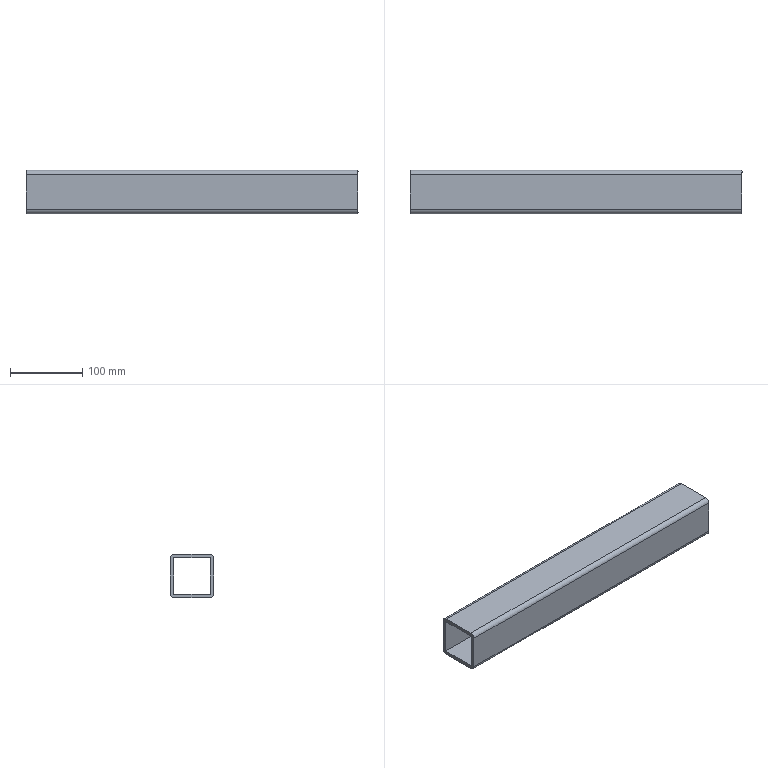Part | STEP file | Positioning_id714_x_t | 1 solid | 14 faces | box 460 x 60 x 60 mm | volume 491785 mm3 | plane 10 | cylinder 4 | commonest cylinder face diameters 12 x4
STEP:
#1=CARTESIAN_POINT('',(0.,0.,0.));
#2=DIRECTION('',(0.,0.,1.));
#3=DIRECTION('',(1.,0.,0.));
#4=AXIS2_PLACEMENT_3D('',#1,#2,#3);
#5=CARTESIAN_POINT('',(-1493.002,-815.,157.466));
#6=VERTEX_POINT('',#5);
#7=CARTESIAN_POINT('',(-1493.002,-765.,157.466));
#8=VERTEX_POINT('',#7);
#9=CARTESIAN_POINT('',(-1493.002,-815.,157.466));
#10=DIRECTION('',(0.,1.,0.));
#11=VECTOR('',#10,1.);
#12=LINE('',#9,#11);
#13=CARTESIAN_POINT('',(-1493.002,-200.,108.466));
#14=DIRECTION('',(1.,0.,0.));
#15=DIRECTION('',(0.,0.,1.));
#16=AXIS2_PLACEMENT_3D('',#13,#14,#15);
#17=PLANE('',#16);
#18=CARTESIAN_POINT('',(49.,615.));
#19=DIRECTION('',(0.,-1.));
#20=VECTOR('',#19,1.);
#21=LINE('',#18,#20);
#22=(GEOMETRIC_REPRESENTATION_CONTEXT(2)PARAMETRIC_REPRESENTATION_CONTEXT()REPRESENTATION_CONTEXT('',''));
#23=DEFINITIONAL_REPRESENTATION('',(#21),#22);
#24=PCURVE('',#17,#23);
#25=CARTESIAN_POINT('',(-1148.002,-815.,157.466));
#26=DIRECTION('',(0.,0.,1.));
#27=DIRECTION('',(0.,1.,0.));
#28=AXIS2_PLACEMENT_3D('',#25,#26,#27);
#29=PLANE('',#28);
#30=CARTESIAN_POINT('',(0.,345.));
#31=DIRECTION('',(1.,0.));
#32=VECTOR('',#31,1.);
#33=LINE('',#30,#32);
#34=(GEOMETRIC_REPRESENTATION_CONTEXT(2)PARAMETRIC_REPRESENTATION_CONTEXT()REPRESENTATION_CONTEXT('',''));
#35=DEFINITIONAL_REPRESENTATION('',(#33),#34);
#36=PCURVE('',#29,#35);
#37=SURFACE_CURVE('',#12,(#24,#36),.PCURVE_S1.);
#38=EDGE_CURVE('',#6,#8,#37,.T.);
#39=ORIENTED_EDGE('',*,*,#38,.F.);
#40=CARTESIAN_POINT('',(-1493.002,-815.,107.466));
#41=VERTEX_POINT('',#40);
#42=CARTESIAN_POINT('',(-1493.002,-815.,107.466));
#43=DIRECTION('',(0.,0.,1.));
#44=VECTOR('',#43,1.);
#45=LINE('',#42,#44);
#46=CARTESIAN_POINT('',(-1.,615.));
#47=DIRECTION('',(1.,0.));
#48=VECTOR('',#47,1.);
#49=LINE('',#46,#48);
#50=(GEOMETRIC_REPRESENTATION_CONTEXT(2)PARAMETRIC_REPRESENTATION_CONTEXT()REPRESENTATION_CONTEXT('',''));
#51=DEFINITIONAL_REPRESENTATION('',(#49),#50);
#52=PCURVE('',#17,#51);
#53=CARTESIAN_POINT('',(-1148.002,-815.,132.466));
#54=DIRECTION('',(0.,-1.,0.));
#55=DIRECTION('',(0.,0.,1.));
#56=AXIS2_PLACEMENT_3D('',#53,#54,#55);
#57=PLANE('',#56);
#58=CARTESIAN_POINT('',(-25.,345.));
#59=DIRECTION('',(1.,0.));
#60=VECTOR('',#59,1.);
#61=LINE('',#58,#60);
#62=(GEOMETRIC_REPRESENTATION_CONTEXT(2)PARAMETRIC_REPRESENTATION_CONTEXT()REPRESENTATION_CONTEXT('',''));
#63=DEFINITIONAL_REPRESENTATION('',(#61),#62);
#64=PCURVE('',#57,#63);
#65=SURFACE_CURVE('',#45,(#52,#64),.PCURVE_S1.);
#66=EDGE_CURVE('',#41,#6,#65,.T.);
#67=ORIENTED_EDGE('',*,*,#66,.F.);
#68=CARTESIAN_POINT('',(-1493.002,-765.,107.466));
#69=VERTEX_POINT('',#68);
#70=CARTESIAN_POINT('',(-1493.002,-765.,107.466));
#71=DIRECTION('',(0.,-1.,0.));
#72=VECTOR('',#71,1.);
#73=LINE('',#70,#72);
#74=CARTESIAN_POINT('',(-1.,565.));
#75=DIRECTION('',(0.,1.));
#76=VECTOR('',#75,1.);
#77=LINE('',#74,#76);
#78=(GEOMETRIC_REPRESENTATION_CONTEXT(2)PARAMETRIC_REPRESENTATION_CONTEXT()REPRESENTATION_CONTEXT('',''));
#79=DEFINITIONAL_REPRESENTATION('',(#77),#78);
#80=PCURVE('',#17,#79);
#81=CARTESIAN_POINT('',(-1148.002,-815.,107.466));
#82=DIRECTION('',(0.,0.,-1.));
#83=DIRECTION('',(0.,-1.,0.));
#84=AXIS2_PLACEMENT_3D('',#81,#82,#83);
#85=PLANE('',#84);
#86=CARTESIAN_POINT('',(-50.,345.));
#87=DIRECTION('',(1.,0.));
#88=VECTOR('',#87,1.);
#89=LINE('',#86,#88);
#90=(GEOMETRIC_REPRESENTATION_CONTEXT(2)PARAMETRIC_REPRESENTATION_CONTEXT()REPRESENTATION_CONTEXT('',''));
#91=DEFINITIONAL_REPRESENTATION('',(#89),#90);
#92=PCURVE('',#85,#91);
#93=SURFACE_CURVE('',#73,(#80,#92),.PCURVE_S1.);
#94=EDGE_CURVE('',#69,#41,#93,.T.);
#95=ORIENTED_EDGE('',*,*,#94,.F.);
#96=CARTESIAN_POINT('',(-1493.002,-765.,157.466));
#97=DIRECTION('',(0.,0.,-1.));
#98=VECTOR('',#97,1.);
#99=LINE('',#96,#98);
#100=CARTESIAN_POINT('',(49.,565.));
#101=DIRECTION('',(-1.,0.));
#102=VECTOR('',#101,1.);
#103=LINE('',#100,#102);
#104=(GEOMETRIC_REPRESENTATION_CONTEXT(2)PARAMETRIC_REPRESENTATION_CONTEXT()REPRESENTATION_CONTEXT('',''));
#105=DEFINITIONAL_REPRESENTATION('',(#103),#104);
#106=PCURVE('',#17,#105);
#107=CARTESIAN_POINT('',(-1148.002,-765.,132.466));
#108=DIRECTION('',(0.,1.,0.));
#109=DIRECTION('',(0.,0.,-1.));
#110=AXIS2_PLACEMENT_3D('',#107,#108,#109);
#111=PLANE('',#110);
#112=CARTESIAN_POINT('',(-25.,345.));
#113=DIRECTION('',(1.,0.));
#114=VECTOR('',#113,1.);
#115=LINE('',#112,#114);
#116=(GEOMETRIC_REPRESENTATION_CONTEXT(2)PARAMETRIC_REPRESENTATION_CONTEXT()REPRESENTATION_CONTEXT('',''));
#117=DEFINITIONAL_REPRESENTATION('',(#115),#116);
#118=PCURVE('',#111,#117);
#119=SURFACE_CURVE('',#99,(#106,#118),.PCURVE_S1.);
#120=EDGE_CURVE('',#8,#69,#119,.T.);
#121=ORIENTED_EDGE('',*,*,#120,.F.);
#122=EDGE_LOOP('',(#39,#67,#95,#121));
#123=FACE_BOUND('',#122,.T.);
#124=CARTESIAN_POINT('',(-1493.002,-760.,108.466));
#125=VERTEX_POINT('',#124);
#126=CARTESIAN_POINT('',(-1493.002,-766.,102.466));
#127=VERTEX_POINT('',#126);
#128=CARTESIAN_POINT('',(-1493.002,-766.,108.466));
#129=DIRECTION('',(-1.,0.,0.));
#130=DIRECTION('',(0.,1.,0.));
#131=AXIS2_PLACEMENT_3D('',#128,#129,#130);
#132=CIRCLE('',#131,6.);
#133=CARTESIAN_POINT('',(0.,560.));
#134=CARTESIAN_POINT('',(-10.392,560.));
#135=CARTESIAN_POINT('',(-5.196,569.));
#136=CARTESIAN_POINT('',(0.,578.));
#137=CARTESIAN_POINT('',(5.196,569.));
#138=CARTESIAN_POINT('',(10.392,560.));
#139=CARTESIAN_POINT('',(0.,560.));
#140=(BOUNDED_CURVE()B_SPLINE_CURVE(2,(#133,#134,#135,#136,#137,#138,#139),.UNSPECIFIED.,.T.,.F.)B_SPLINE_CURVE_WITH_KNOTS((1,2,2,2,2,1),(-2.094,0.,2.094,4.189,6.283,8.378),.UNSPECIFIED.)CURVE()GEOMETRIC_REPRESENTATION_ITEM()RATIONAL_B_SPLINE_CURVE((1.,0.5,1.,0.5,1.,0.5,1.))REPRESENTATION_ITEM(''));
#141=(GEOMETRIC_REPRESENTATION_CONTEXT(2)PARAMETRIC_REPRESENTATION_CONTEXT()REPRESENTATION_CONTEXT('',''));
#142=DEFINITIONAL_REPRESENTATION('',(#140),#141);
#143=PCURVE('',#17,#142);
#144=CARTESIAN_POINT('',(-1148.002,-766.,108.466));
#145=DIRECTION('',(-1.,0.,0.));
#146=DIRECTION('',(0.,0.,1.));
#147=AXIS2_PLACEMENT_3D('',#144,#145,#146);
#148=CYLINDRICAL_SURFACE('',#147,6.);
#149=CARTESIAN_POINT('',(1.571,345.));
#150=DIRECTION('',(1.,0.));
#151=VECTOR('',#150,1.);
#152=LINE('',#149,#151);
#153=(GEOMETRIC_REPRESENTATION_CONTEXT(2)PARAMETRIC_REPRESENTATION_CONTEXT()REPRESENTATION_CONTEXT('',''));
#154=DEFINITIONAL_REPRESENTATION('',(#152),#153);
#155=PCURVE('',#148,#154);
#156=SURFACE_CURVE('',#132,(#143,#155),.PCURVE_S1.);
#157=EDGE_CURVE('',#125,#127,#156,.T.);
#158=ORIENTED_EDGE('',*,*,#157,.T.);
#159=CARTESIAN_POINT('',(-1493.002,-814.,102.466));
#160=VERTEX_POINT('',#159);
#161=CARTESIAN_POINT('',(-1493.002,-766.,102.466));
#162=DIRECTION('',(0.,-1.,0.));
#163=VECTOR('',#162,1.);
#164=LINE('',#161,#163);
#165=CARTESIAN_POINT('',(-6.,566.));
#166=DIRECTION('',(0.,1.));
#167=VECTOR('',#166,1.);
#168=LINE('',#165,#167);
#169=(GEOMETRIC_REPRESENTATION_CONTEXT(2)PARAMETRIC_REPRESENTATION_CONTEXT()REPRESENTATION_CONTEXT('',''));
#170=DEFINITIONAL_REPRESENTATION('',(#168),#169);
#171=PCURVE('',#17,#170);
#172=CARTESIAN_POINT('',(-1148.002,-820.,102.466));
#173=DIRECTION('',(0.,0.,-1.));
#174=DIRECTION('',(0.,-1.,0.));
#175=AXIS2_PLACEMENT_3D('',#172,#173,#174);
#176=PLANE('',#175);
#177=CARTESIAN_POINT('',(-54.,345.));
#178=DIRECTION('',(1.,0.));
#179=VECTOR('',#178,1.);
#180=LINE('',#177,#179);
#181=(GEOMETRIC_REPRESENTATION_CONTEXT(2)PARAMETRIC_REPRESENTATION_CONTEXT()REPRESENTATION_CONTEXT('',''));
#182=DEFINITIONAL_REPRESENTATION('',(#180),#181);
#183=PCURVE('',#176,#182);
#184=SURFACE_CURVE('',#164,(#171,#183),.PCURVE_S1.);
#185=EDGE_CURVE('',#127,#160,#184,.T.);
#186=ORIENTED_EDGE('',*,*,#185,.T.);
#187=CARTESIAN_POINT('',(-1493.002,-820.,108.466));
#188=VERTEX_POINT('',#187);
#189=CARTESIAN_POINT('',(-1493.002,-814.,108.466));
#190=DIRECTION('',(-1.,0.,0.));
#191=DIRECTION('',(0.,0.,-1.));
#192=AXIS2_PLACEMENT_3D('',#189,#190,#191);
#193=CIRCLE('',#192,6.);
#194=CARTESIAN_POINT('',(-6.,614.));
#195=CARTESIAN_POINT('',(-6.,624.392));
#196=CARTESIAN_POINT('',(3.,619.196));
#197=CARTESIAN_POINT('',(12.,614.));
#198=CARTESIAN_POINT('',(3.,608.804));
#199=CARTESIAN_POINT('',(-6.,603.608));
#200=CARTESIAN_POINT('',(-6.,614.));
#201=(BOUNDED_CURVE()B_SPLINE_CURVE(2,(#194,#195,#196,#197,#198,#199,#200),.UNSPECIFIED.,.T.,.F.)B_SPLINE_CURVE_WITH_KNOTS((1,2,2,2,2,1),(-2.094,0.,2.094,4.189,6.283,8.378),.UNSPECIFIED.)CURVE()GEOMETRIC_REPRESENTATION_ITEM()RATIONAL_B_SPLINE_CURVE((1.,0.5,1.,0.5,1.,0.5,1.))REPRESENTATION_ITEM(''));
#202=(GEOMETRIC_REPRESENTATION_CONTEXT(2)PARAMETRIC_REPRESENTATION_CONTEXT()REPRESENTATION_CONTEXT('',''));
#203=DEFINITIONAL_REPRESENTATION('',(#201),#202);
#204=PCURVE('',#17,#203);
#205=CARTESIAN_POINT('',(-1148.002,-814.,108.466));
#206=DIRECTION('',(1.,0.,0.));
#207=DIRECTION('',(0.,0.,-1.));
#208=AXIS2_PLACEMENT_3D('',#205,#206,#207);
#209=CYLINDRICAL_SURFACE('',#208,6.);
#210=CARTESIAN_POINT('',(6.283,-345.));
#211=DIRECTION('',(-1.,0.));
#212=VECTOR('',#211,1.);
#213=LINE('',#210,#212);
#214=(GEOMETRIC_REPRESENTATION_CONTEXT(2)PARAMETRIC_REPRESENTATION_CONTEXT()REPRESENTATION_CONTEXT('',''));
#215=DEFINITIONAL_REPRESENTATION('',(#213),#214);
#216=PCURVE('',#209,#215);
#217=SURFACE_CURVE('',#193,(#204,#216),.PCURVE_S1.);
#218=EDGE_CURVE('',#160,#188,#217,.T.);
#219=ORIENTED_EDGE('',*,*,#218,.T.);
#220=CARTESIAN_POINT('',(-1493.002,-820.,156.466));
#221=VERTEX_POINT('',#220);
#222=CARTESIAN_POINT('',(-1493.002,-820.,108.466));
#223=DIRECTION('',(0.,0.,1.));
#224=VECTOR('',#223,1.);
#225=LINE('',#222,#224);
#226=CARTESIAN_POINT('',(0.,620.));
#227=DIRECTION('',(1.,0.));
#228=VECTOR('',#227,1.);
#229=LINE('',#226,#228);
#230=(GEOMETRIC_REPRESENTATION_CONTEXT(2)PARAMETRIC_REPRESENTATION_CONTEXT()REPRESENTATION_CONTEXT('',''));
#231=DEFINITIONAL_REPRESENTATION('',(#229),#230);
#232=PCURVE('',#17,#231);
#233=CARTESIAN_POINT('',(-1148.002,-820.,132.466));
#234=DIRECTION('',(0.,-1.,0.));
#235=DIRECTION('',(0.,0.,1.));
#236=AXIS2_PLACEMENT_3D('',#233,#234,#235);
#237=PLANE('',#236);
#238=CARTESIAN_POINT('',(-24.,345.));
#239=DIRECTION('',(1.,0.));
#240=VECTOR('',#239,1.);
#241=LINE('',#238,#240);
#242=(GEOMETRIC_REPRESENTATION_CONTEXT(2)PARAMETRIC_REPRESENTATION_CONTEXT()REPRESENTATION_CONTEXT('',''));
#243=DEFINITIONAL_REPRESENTATION('',(#241),#242);
#244=PCURVE('',#237,#243);
#245=SURFACE_CURVE('',#225,(#232,#244),.PCURVE_S1.);
#246=EDGE_CURVE('',#188,#221,#245,.T.);
#247=ORIENTED_EDGE('',*,*,#246,.T.);
#248=CARTESIAN_POINT('',(-1493.002,-814.,162.466));
#249=VERTEX_POINT('',#248);
#250=CARTESIAN_POINT('',(-1493.002,-814.,156.466));
#251=DIRECTION('',(-1.,0.,0.));
#252=DIRECTION('',(0.,-1.,0.));
#253=AXIS2_PLACEMENT_3D('',#250,#251,#252);
#254=CIRCLE('',#253,6.);
#255=CARTESIAN_POINT('',(48.,620.));
#256=CARTESIAN_POINT('',(58.392,620.));
#257=CARTESIAN_POINT('',(53.196,611.));
#258=CARTESIAN_POINT('',(48.,602.));
#259=CARTESIAN_POINT('',(42.804,611.));
#260=CARTESIAN_POINT('',(37.608,620.));
#261=CARTESIAN_POINT('',(48.,620.));
#262=(BOUNDED_CURVE()B_SPLINE_CURVE(2,(#255,#256,#257,#258,#259,#260,#261),.UNSPECIFIED.,.T.,.F.)B_SPLINE_CURVE_WITH_KNOTS((1,2,2,2,2,1),(-2.094,0.,2.094,4.189,6.283,8.378),.UNSPECIFIED.)CURVE()GEOMETRIC_REPRESENTATION_ITEM()RATIONAL_B_SPLINE_CURVE((1.,0.5,1.,0.5,1.,0.5,1.))REPRESENTATION_ITEM(''));
#263=(GEOMETRIC_REPRESENTATION_CONTEXT(2)PARAMETRIC_REPRESENTATION_CONTEXT()REPRESENTATION_CONTEXT('',''));
#264=DEFINITIONAL_REPRESENTATION('',(#262),#263);
#265=PCURVE('',#17,#264);
#266=CARTESIAN_POINT('',(-1148.002,-814.,156.466));
#267=DIRECTION('',(-1.,0.,0.));
#268=DIRECTION('',(0.,0.,1.));
#269=AXIS2_PLACEMENT_3D('',#266,#267,#268);
#270=CYLINDRICAL_SURFACE('',#269,6.);
#271=CARTESIAN_POINT('',(4.712,345.));
#272=DIRECTION('',(1.,0.));
#273=VECTOR('',#272,1.);
#274=LINE('',#271,#273);
#275=(GEOMETRIC_REPRESENTATION_CONTEXT(2)PARAMETRIC_REPRESENTATION_CONTEXT()REPRESENTATION_CONTEXT('',''));
#276=DEFINITIONAL_REPRESENTATION('',(#274),#275);
#277=PCURVE('',#270,#276);
#278=SURFACE_CURVE('',#254,(#265,#277),.PCURVE_S1.);
#279=EDGE_CURVE('',#221,#249,#278,.T.);
#280=ORIENTED_EDGE('',*,*,#279,.T.);
#281=CARTESIAN_POINT('',(-1493.002,-766.,162.466));
#282=VERTEX_POINT('',#281);
#283=CARTESIAN_POINT('',(-1493.002,-814.,162.466));
#284=DIRECTION('',(0.,1.,0.));
#285=VECTOR('',#284,1.);
#286=LINE('',#283,#285);
#287=CARTESIAN_POINT('',(54.,614.));
#288=DIRECTION('',(0.,-1.));
#289=VECTOR('',#288,1.);
#290=LINE('',#287,#289);
#291=(GEOMETRIC_REPRESENTATION_CONTEXT(2)PARAMETRIC_REPRESENTATION_CONTEXT()REPRESENTATION_CONTEXT('',''));
#292=DEFINITIONAL_REPRESENTATION('',(#290),#291);
#293=PCURVE('',#17,#292);
#294=CARTESIAN_POINT('',(-1148.002,-820.,162.466));
#295=DIRECTION('',(0.,0.,1.));
#296=DIRECTION('',(0.,1.,0.));
#297=AXIS2_PLACEMENT_3D('',#294,#295,#296);
#298=PLANE('',#297);
#299=CARTESIAN_POINT('',(6.,345.));
#300=DIRECTION('',(1.,0.));
#301=VECTOR('',#300,1.);
#302=LINE('',#299,#301);
#303=(GEOMETRIC_REPRESENTATION_CONTEXT(2)PARAMETRIC_REPRESENTATION_CONTEXT()REPRESENTATION_CONTEXT('',''));
#304=DEFINITIONAL_REPRESENTATION('',(#302),#303);
#305=PCURVE('',#298,#304);
#306=SURFACE_CURVE('',#286,(#293,#305),.PCURVE_S1.);
#307=EDGE_CURVE('',#249,#282,#306,.T.);
#308=ORIENTED_EDGE('',*,*,#307,.T.);
#309=CARTESIAN_POINT('',(-1493.002,-760.,156.466));
#310=VERTEX_POINT('',#309);
#311=CARTESIAN_POINT('',(-1493.002,-766.,156.466));
#312=DIRECTION('',(-1.,0.,0.));
#313=DIRECTION('',(0.,0.,1.));
#314=AXIS2_PLACEMENT_3D('',#311,#312,#313);
#315=CIRCLE('',#314,6.);
#316=CARTESIAN_POINT('',(54.,566.));
#317=CARTESIAN_POINT('',(54.,555.608));
#318=CARTESIAN_POINT('',(45.,560.804));
#319=CARTESIAN_POINT('',(36.,566.));
#320=CARTESIAN_POINT('',(45.,571.196));
#321=CARTESIAN_POINT('',(54.,576.392));
#322=CARTESIAN_POINT('',(54.,566.));
#323=(BOUNDED_CURVE()B_SPLINE_CURVE(2,(#316,#317,#318,#319,#320,#321,#322),.UNSPECIFIED.,.T.,.F.)B_SPLINE_CURVE_WITH_KNOTS((1,2,2,2,2,1),(-2.094,0.,2.094,4.189,6.283,8.378),.UNSPECIFIED.)CURVE()GEOMETRIC_REPRESENTATION_ITEM()RATIONAL_B_SPLINE_CURVE((1.,0.5,1.,0.5,1.,0.5,1.))REPRESENTATION_ITEM(''));
#324=(GEOMETRIC_REPRESENTATION_CONTEXT(2)PARAMETRIC_REPRESENTATION_CONTEXT()REPRESENTATION_CONTEXT('',''));
#325=DEFINITIONAL_REPRESENTATION('',(#323),#324);
#326=PCURVE('',#17,#325);
#327=CARTESIAN_POINT('',(-1148.002,-766.,156.466));
#328=DIRECTION('',(1.,0.,0.));
#329=DIRECTION('',(0.,0.,-1.));
#330=AXIS2_PLACEMENT_3D('',#327,#328,#329);
#331=CYLINDRICAL_SURFACE('',#330,6.);
#332=CARTESIAN_POINT('',(3.142,-345.));
#333=DIRECTION('',(-1.,0.));
#334=VECTOR('',#333,1.);
#335=LINE('',#332,#334);
#336=(GEOMETRIC_REPRESENTATION_CONTEXT(2)PARAMETRIC_REPRESENTATION_CONTEXT()REPRESENTATION_CONTEXT('',''));
#337=DEFINITIONAL_REPRESENTATION('',(#335),#336);
#338=PCURVE('',#331,#337);
#339=SURFACE_CURVE('',#315,(#326,#338),.PCURVE_S1.);
#340=EDGE_CURVE('',#282,#310,#339,.T.);
#341=ORIENTED_EDGE('',*,*,#340,.T.);
#342=CARTESIAN_POINT('',(-1493.002,-760.,156.466));
#343=DIRECTION('',(0.,0.,-1.));
#344=VECTOR('',#343,1.);
#345=LINE('',#342,#344);
#346=CARTESIAN_POINT('',(48.,560.));
#347=DIRECTION('',(-1.,0.));
#348=VECTOR('',#347,1.);
#349=LINE('',#346,#348);
#350=(GEOMETRIC_REPRESENTATION_CONTEXT(2)PARAMETRIC_REPRESENTATION_CONTEXT()REPRESENTATION_CONTEXT('',''));
#351=DEFINITIONAL_REPRESENTATION('',(#349),#350);
#352=PCURVE('',#17,#351);
#353=CARTESIAN_POINT('',(-1148.002,-760.,132.466));
#354=DIRECTION('',(0.,1.,0.));
#355=DIRECTION('',(0.,0.,-1.));
#356=AXIS2_PLACEMENT_3D('',#353,#354,#355);
#357=PLANE('',#356);
#358=CARTESIAN_POINT('',(-24.,345.));
#359=DIRECTION('',(1.,0.));
#360=VECTOR('',#359,1.);
#361=LINE('',#358,#360);
#362=(GEOMETRIC_REPRESENTATION_CONTEXT(2)PARAMETRIC_REPRESENTATION_CONTEXT()REPRESENTATION_CONTEXT('',''));
#363=DEFINITIONAL_REPRESENTATION('',(#361),#362);
#364=PCURVE('',#357,#363);
#365=SURFACE_CURVE('',#345,(#352,#364),.PCURVE_S1.);
#366=EDGE_CURVE('',#310,#125,#365,.T.);
#367=ORIENTED_EDGE('',*,*,#366,.T.);
#368=EDGE_LOOP('',(#158,#186,#219,#247,#280,#308,#341,#367));
#369=FACE_BOUND('',#368,.T.);
#370=ADVANCED_FACE('',(#123,#369),#17,.F.);
#371=CARTESIAN_POINT('',(-1033.002,-815.,107.466));
#372=VERTEX_POINT('',#371);
#373=CARTESIAN_POINT('',(-1033.002,-765.,107.466));
#374=VERTEX_POINT('',#373);
#375=CARTESIAN_POINT('',(-1033.002,-815.,107.466));
#376=DIRECTION('',(0.,1.,0.));
#377=VECTOR('',#376,1.);
#378=LINE('',#375,#377);
#379=CARTESIAN_POINT('',(-1033.002,-1380.,108.466));
#380=DIRECTION('',(-1.,0.,0.));
#381=DIRECTION('',(0.,0.,-1.));
#382=AXIS2_PLACEMENT_3D('',#379,#380,#381);
#383=PLANE('',#382);
#384=CARTESIAN_POINT('',(1.,-565.));
#385=DIRECTION('',(0.,-1.));
#386=VECTOR('',#385,1.);
#387=LINE('',#384,#386);
#388=(GEOMETRIC_REPRESENTATION_CONTEXT(2)PARAMETRIC_REPRESENTATION_CONTEXT()REPRESENTATION_CONTEXT('',''));
#389=DEFINITIONAL_REPRESENTATION('',(#387),#388);
#390=PCURVE('',#383,#389);
#391=CARTESIAN_POINT('',(0.,-115.));
#392=DIRECTION('',(-1.,0.));
#393=VECTOR('',#392,1.);
#394=LINE('',#391,#393);
#395=(GEOMETRIC_REPRESENTATION_CONTEXT(2)PARAMETRIC_REPRESENTATION_CONTEXT()REPRESENTATION_CONTEXT('',''));
#396=DEFINITIONAL_REPRESENTATION('',(#394),#395);
#397=PCURVE('',#85,#396);
#398=SURFACE_CURVE('',#378,(#390,#397),.PCURVE_S1.);
#399=EDGE_CURVE('',#372,#374,#398,.T.);
#400=ORIENTED_EDGE('',*,*,#399,.F.);
#401=CARTESIAN_POINT('',(-1033.002,-815.,157.466));
#402=VERTEX_POINT('',#401);
#403=CARTESIAN_POINT('',(-1033.002,-815.,157.466));
#404=DIRECTION('',(0.,0.,-1.));
#405=VECTOR('',#404,1.);
#406=LINE('',#403,#405);
#407=CARTESIAN_POINT('',(-49.,-565.));
#408=DIRECTION('',(1.,0.));
#409=VECTOR('',#408,1.);
#410=LINE('',#407,#409);
#411=(GEOMETRIC_REPRESENTATION_CONTEXT(2)PARAMETRIC_REPRESENTATION_CONTEXT()REPRESENTATION_CONTEXT('',''));
#412=DEFINITIONAL_REPRESENTATION('',(#410),#411);
#413=PCURVE('',#383,#412);
#414=CARTESIAN_POINT('',(25.,-115.));
#415=DIRECTION('',(-1.,0.));
#416=VECTOR('',#415,1.);
#417=LINE('',#414,#416);
#418=(GEOMETRIC_REPRESENTATION_CONTEXT(2)PARAMETRIC_REPRESENTATION_CONTEXT()REPRESENTATION_CONTEXT('',''));
#419=DEFINITIONAL_REPRESENTATION('',(#417),#418);
#420=PCURVE('',#57,#419);
#421=SURFACE_CURVE('',#406,(#413,#420),.PCURVE_S1.);
#422=EDGE_CURVE('',#402,#372,#421,.T.);
#423=ORIENTED_EDGE('',*,*,#422,.F.);
#424=CARTESIAN_POINT('',(-1033.002,-765.,157.466));
#425=VERTEX_POINT('',#424);
#426=CARTESIAN_POINT('',(-1033.002,-765.,157.466));
#427=DIRECTION('',(0.,-1.,0.));
#428=VECTOR('',#427,1.);
#429=LINE('',#426,#428);
#430=CARTESIAN_POINT('',(-49.,-615.));
#431=DIRECTION('',(0.,1.));
#432=VECTOR('',#431,1.);
#433=LINE('',#430,#432);
#434=(GEOMETRIC_REPRESENTATION_CONTEXT(2)PARAMETRIC_REPRESENTATION_CONTEXT()REPRESENTATION_CONTEXT('',''));
#435=DEFINITIONAL_REPRESENTATION('',(#433),#434);
#436=PCURVE('',#383,#435);
#437=CARTESIAN_POINT('',(50.,-115.));
#438=DIRECTION('',(-1.,0.));
#439=VECTOR('',#438,1.);
#440=LINE('',#437,#439);
#441=(GEOMETRIC_REPRESENTATION_CONTEXT(2)PARAMETRIC_REPRESENTATION_CONTEXT()REPRESENTATION_CONTEXT('',''));
#442=DEFINITIONAL_REPRESENTATION('',(#440),#441);
#443=PCURVE('',#29,#442);
#444=SURFACE_CURVE('',#429,(#436,#443),.PCURVE_S1.);
#445=EDGE_CURVE('',#425,#402,#444,.T.);
#446=ORIENTED_EDGE('',*,*,#445,.F.);
#447=CARTESIAN_POINT('',(-1033.002,-765.,107.466));
#448=DIRECTION('',(0.,0.,1.));
#449=VECTOR('',#448,1.);
#450=LINE('',#447,#449);
#451=CARTESIAN_POINT('',(1.,-615.));
#452=DIRECTION('',(-1.,0.));
#453=VECTOR('',#452,1.);
#454=LINE('',#451,#453);
#455=(GEOMETRIC_REPRESENTATION_CONTEXT(2)PARAMETRIC_REPRESENTATION_CONTEXT()REPRESENTATION_CONTEXT('',''));
#456=DEFINITIONAL_REPRESENTATION('',(#454),#455);
#457=PCURVE('',#383,#456);
#458=CARTESIAN_POINT('',(25.,-115.));
#459=DIRECTION('',(-1.,0.));
#460=VECTOR('',#459,1.);
#461=LINE('',#458,#460);
#462=(GEOMETRIC_REPRESENTATION_CONTEXT(2)PARAMETRIC_REPRESENTATION_CONTEXT()REPRESENTATION_CONTEXT('',''));
#463=DEFINITIONAL_REPRESENTATION('',(#461),#462);
#464=PCURVE('',#111,#463);
#465=SURFACE_CURVE('',#450,(#457,#464),.PCURVE_S1.);
#466=EDGE_CURVE('',#374,#425,#465,.T.);
#467=ORIENTED_EDGE('',*,*,#466,.F.);
#468=EDGE_LOOP('',(#400,#423,#446,#467));
#469=FACE_BOUND('',#468,.T.);
#470=CARTESIAN_POINT('',(-1033.002,-766.,102.466));
#471=VERTEX_POINT('',#470);
#472=CARTESIAN_POINT('',(-1033.002,-760.,108.466));
#473=VERTEX_POINT('',#472);
#474=CARTESIAN_POINT('',(-1033.002,-766.,108.466));
#475=DIRECTION('',(1.,0.,0.));
#476=DIRECTION('',(0.,0.,-1.));
#477=AXIS2_PLACEMENT_3D('',#474,#475,#476);
#478=CIRCLE('',#477,6.);
#479=CARTESIAN_POINT('',(6.,-614.));
#480=CARTESIAN_POINT('',(6.,-624.392));
#481=CARTESIAN_POINT('',(-3.,-619.196));
#482=CARTESIAN_POINT('',(-12.,-614.));
#483=CARTESIAN_POINT('',(-3.,-608.804));
#484=CARTESIAN_POINT('',(6.,-603.608));
#485=CARTESIAN_POINT('',(6.,-614.));
#486=(BOUNDED_CURVE()B_SPLINE_CURVE(2,(#479,#480,#481,#482,#483,#484,#485),.UNSPECIFIED.,.T.,.F.)B_SPLINE_CURVE_WITH_KNOTS((1,2,2,2,2,1),(-2.094,0.,2.094,4.189,6.283,8.378),.UNSPECIFIED.)CURVE()GEOMETRIC_REPRESENTATION_ITEM()RATIONAL_B_SPLINE_CURVE((1.,0.5,1.,0.5,1.,0.5,1.))REPRESENTATION_ITEM(''));
#487=(GEOMETRIC_REPRESENTATION_CONTEXT(2)PARAMETRIC_REPRESENTATION_CONTEXT()REPRESENTATION_CONTEXT('',''));
#488=DEFINITIONAL_REPRESENTATION('',(#486),#487);
#489=PCURVE('',#383,#488);
#490=CARTESIAN_POINT('',(3.142,-115.));
#491=DIRECTION('',(-1.,0.));
#492=VECTOR('',#491,1.);
#493=LINE('',#490,#492);
#494=(GEOMETRIC_REPRESENTATION_CONTEXT(2)PARAMETRIC_REPRESENTATION_CONTEXT()REPRESENTATION_CONTEXT('',''));
#495=DEFINITIONAL_REPRESENTATION('',(#493),#494);
#496=PCURVE('',#148,#495);
#497=SURFACE_CURVE('',#478,(#489,#496),.PCURVE_S1.);
#498=EDGE_CURVE('',#471,#473,#497,.T.);
#499=ORIENTED_EDGE('',*,*,#498,.T.);
#500=CARTESIAN_POINT('',(-1033.002,-760.,156.466));
#501=VERTEX_POINT('',#500);
#502=CARTESIAN_POINT('',(-1033.002,-760.,156.466));
#503=DIRECTION('',(0.,0.,-1.));
#504=VECTOR('',#503,1.);
#505=LINE('',#502,#504);
#506=CARTESIAN_POINT('',(-48.,-620.));
#507=DIRECTION('',(1.,0.));
#508=VECTOR('',#507,1.);
#509=LINE('',#506,#508);
#510=(GEOMETRIC_REPRESENTATION_CONTEXT(2)PARAMETRIC_REPRESENTATION_CONTEXT()REPRESENTATION_CONTEXT('',''));
#511=DEFINITIONAL_REPRESENTATION('',(#509),#510);
#512=PCURVE('',#383,#511);
#513=CARTESIAN_POINT('',(-24.,-115.));
#514=DIRECTION('',(1.,0.));
#515=VECTOR('',#514,1.);
#516=LINE('',#513,#515);
#517=(GEOMETRIC_REPRESENTATION_CONTEXT(2)PARAMETRIC_REPRESENTATION_CONTEXT()REPRESENTATION_CONTEXT('',''));
#518=DEFINITIONAL_REPRESENTATION('',(#516),#517);
#519=PCURVE('',#357,#518);
#520=SURFACE_CURVE('',#505,(#512,#519),.PCURVE_S1.);
#521=EDGE_CURVE('',#501,#473,#520,.T.);
#522=ORIENTED_EDGE('',*,*,#521,.F.);
#523=CARTESIAN_POINT('',(-1033.002,-766.,162.466));
#524=VERTEX_POINT('',#523);
#525=CARTESIAN_POINT('',(-1033.002,-766.,156.466));
#526=DIRECTION('',(1.,0.,0.));
#527=DIRECTION('',(0.,1.,0.));
#528=AXIS2_PLACEMENT_3D('',#525,#526,#527);
#529=CIRCLE('',#528,6.);
#530=CARTESIAN_POINT('',(-48.,-620.));
#531=CARTESIAN_POINT('',(-58.392,-620.));
#532=CARTESIAN_POINT('',(-53.196,-611.));
#533=CARTESIAN_POINT('',(-48.,-602.));
#534=CARTESIAN_POINT('',(-42.804,-611.));
#535=CARTESIAN_POINT('',(-37.608,-620.));
#536=CARTESIAN_POINT('',(-48.,-620.));
#537=(BOUNDED_CURVE()B_SPLINE_CURVE(2,(#530,#531,#532,#533,#534,#535,#536),.UNSPECIFIED.,.T.,.F.)B_SPLINE_CURVE_WITH_KNOTS((1,2,2,2,2,1),(-2.094,0.,2.094,4.189,6.283,8.378),.UNSPECIFIED.)CURVE()GEOMETRIC_REPRESENTATION_ITEM()RATIONAL_B_SPLINE_CURVE((1.,0.5,1.,0.5,1.,0.5,1.))REPRESENTATION_ITEM(''));
#538=(GEOMETRIC_REPRESENTATION_CONTEXT(2)PARAMETRIC_REPRESENTATION_CONTEXT()REPRESENTATION_CONTEXT('',''));
#539=DEFINITIONAL_REPRESENTATION('',(#537),#538);
#540=PCURVE('',#383,#539);
#541=CARTESIAN_POINT('',(1.571,115.));
#542=DIRECTION('',(1.,0.));
#543=VECTOR('',#542,1.);
#544=LINE('',#541,#543);
#545=(GEOMETRIC_REPRESENTATION_CONTEXT(2)PARAMETRIC_REPRESENTATION_CONTEXT()REPRESENTATION_CONTEXT('',''));
#546=DEFINITIONAL_REPRESENTATION('',(#544),#545);
#547=PCURVE('',#331,#546);
#548=SURFACE_CURVE('',#529,(#540,#547),.PCURVE_S1.);
#549=EDGE_CURVE('',#501,#524,#548,.T.);
#550=ORIENTED_EDGE('',*,*,#549,.T.);
#551=CARTESIAN_POINT('',(-1033.002,-814.,162.466));
#552=VERTEX_POINT('',#551);
#553=CARTESIAN_POINT('',(-1033.002,-766.,162.466));
#554=DIRECTION('',(0.,-1.,0.));
#555=VECTOR('',#554,1.);
#556=LINE('',#553,#555);
#557=CARTESIAN_POINT('',(-54.,-614.));
#558=DIRECTION('',(0.,1.));
#559=VECTOR('',#558,1.);
#560=LINE('',#557,#559);
#561=(GEOMETRIC_REPRESENTATION_CONTEXT(2)PARAMETRIC_REPRESENTATION_CONTEXT()REPRESENTATION_CONTEXT('',''));
#562=DEFINITIONAL_REPRESENTATION('',(#560),#561);
#563=PCURVE('',#383,#562);
#564=CARTESIAN_POINT('',(54.,-115.));
#565=DIRECTION('',(-1.,0.));
#566=VECTOR('',#565,1.);
#567=LINE('',#564,#566);
#568=(GEOMETRIC_REPRESENTATION_CONTEXT(2)PARAMETRIC_REPRESENTATION_CONTEXT()REPRESENTATION_CONTEXT('',''));
#569=DEFINITIONAL_REPRESENTATION('',(#567),#568);
#570=PCURVE('',#298,#569);
#571=SURFACE_CURVE('',#556,(#563,#570),.PCURVE_S1.);
#572=EDGE_CURVE('',#524,#552,#571,.T.);
#573=ORIENTED_EDGE('',*,*,#572,.T.);
#574=CARTESIAN_POINT('',(-1033.002,-820.,156.466));
#575=VERTEX_POINT('',#574);
#576=CARTESIAN_POINT('',(-1033.002,-814.,156.466));
#577=DIRECTION('',(1.,0.,0.));
#578=DIRECTION('',(0.,0.,1.));
#579=AXIS2_PLACEMENT_3D('',#576,#577,#578);
#580=CIRCLE('',#579,6.);
#581=CARTESIAN_POINT('',(-54.,-566.));
#582=CARTESIAN_POINT('',(-54.,-555.608));
#583=CARTESIAN_POINT('',(-45.,-560.804));
#584=CARTESIAN_POINT('',(-36.,-566.));
#585=CARTESIAN_POINT('',(-45.,-571.196));
#586=CARTESIAN_POINT('',(-54.,-576.392));
#587=CARTESIAN_POINT('',(-54.,-566.));
#588=(BOUNDED_CURVE()B_SPLINE_CURVE(2,(#581,#582,#583,#584,#585,#586,#587),.UNSPECIFIED.,.T.,.F.)B_SPLINE_CURVE_WITH_KNOTS((1,2,2,2,2,1),(-2.094,0.,2.094,4.189,6.283,8.378),.UNSPECIFIED.)CURVE()GEOMETRIC_REPRESENTATION_ITEM()RATIONAL_B_SPLINE_CURVE((1.,0.5,1.,0.5,1.,0.5,1.))REPRESENTATION_ITEM(''));
#589=(GEOMETRIC_REPRESENTATION_CONTEXT(2)PARAMETRIC_REPRESENTATION_CONTEXT()REPRESENTATION_CONTEXT('',''));
#590=DEFINITIONAL_REPRESENTATION('',(#588),#589);
#591=PCURVE('',#383,#590);
#592=CARTESIAN_POINT('',(6.283,-115.));
#593=DIRECTION('',(-1.,0.));
#594=VECTOR('',#593,1.);
#595=LINE('',#592,#594);
#596=(GEOMETRIC_REPRESENTATION_CONTEXT(2)PARAMETRIC_REPRESENTATION_CONTEXT()REPRESENTATION_CONTEXT('',''));
#597=DEFINITIONAL_REPRESENTATION('',(#595),#596);
#598=PCURVE('',#270,#597);
#599=SURFACE_CURVE('',#580,(#591,#598),.PCURVE_S1.);
#600=EDGE_CURVE('',#552,#575,#599,.T.);
#601=ORIENTED_EDGE('',*,*,#600,.T.);
#602=CARTESIAN_POINT('',(-1033.002,-820.,108.466));
#603=VERTEX_POINT('',#602);
#604=CARTESIAN_POINT('',(-1033.002,-820.,156.466));
#605=DIRECTION('',(0.,0.,-1.));
#606=VECTOR('',#605,1.);
#607=LINE('',#604,#606);
#608=CARTESIAN_POINT('',(-48.,-560.));
#609=DIRECTION('',(1.,0.));
#610=VECTOR('',#609,1.);
#611=LINE('',#608,#610);
#612=(GEOMETRIC_REPRESENTATION_CONTEXT(2)PARAMETRIC_REPRESENTATION_CONTEXT()REPRESENTATION_CONTEXT('',''));
#613=DEFINITIONAL_REPRESENTATION('',(#611),#612);
#614=PCURVE('',#383,#613);
#615=CARTESIAN_POINT('',(24.,-115.));
#616=DIRECTION('',(-1.,0.));
#617=VECTOR('',#616,1.);
#618=LINE('',#615,#617);
#619=(GEOMETRIC_REPRESENTATION_CONTEXT(2)PARAMETRIC_REPRESENTATION_CONTEXT()REPRESENTATION_CONTEXT('',''));
#620=DEFINITIONAL_REPRESENTATION('',(#618),#619);
#621=PCURVE('',#237,#620);
#622=SURFACE_CURVE('',#607,(#614,#621),.PCURVE_S1.);
#623=EDGE_CURVE('',#575,#603,#622,.T.);
#624=ORIENTED_EDGE('',*,*,#623,.T.);
#625=CARTESIAN_POINT('',(-1033.002,-814.,102.466));
#626=VERTEX_POINT('',#625);
#627=CARTESIAN_POINT('',(-1033.002,-814.,108.466));
#628=DIRECTION('',(1.,0.,0.));
#629=DIRECTION('',(0.,-1.,0.));
#630=AXIS2_PLACEMENT_3D('',#627,#628,#629);
#631=CIRCLE('',#630,6.);
#632=CARTESIAN_POINT('',(0.,-560.));
#633=CARTESIAN_POINT('',(10.392,-560.));
#634=CARTESIAN_POINT('',(5.196,-569.));
#635=CARTESIAN_POINT('',(0.,-578.));
#636=CARTESIAN_POINT('',(-5.196,-569.));
#637=CARTESIAN_POINT('',(-10.392,-560.));
#638=CARTESIAN_POINT('',(0.,-560.));
#639=(BOUNDED_CURVE()B_SPLINE_CURVE(2,(#632,#633,#634,#635,#636,#637,#638),.UNSPECIFIED.,.T.,.F.)B_SPLINE_CURVE_WITH_KNOTS((1,2,2,2,2,1),(-2.094,0.,2.094,4.189,6.283,8.378),.UNSPECIFIED.)CURVE()GEOMETRIC_REPRESENTATION_ITEM()RATIONAL_B_SPLINE_CURVE((1.,0.5,1.,0.5,1.,0.5,1.))REPRESENTATION_ITEM(''));
#640=(GEOMETRIC_REPRESENTATION_CONTEXT(2)PARAMETRIC_REPRESENTATION_CONTEXT()REPRESENTATION_CONTEXT('',''));
#641=DEFINITIONAL_REPRESENTATION('',(#639),#640);
#642=PCURVE('',#383,#641);
#643=CARTESIAN_POINT('',(4.712,115.));
#644=DIRECTION('',(1.,0.));
#645=VECTOR('',#644,1.);
#646=LINE('',#643,#645);
#647=(GEOMETRIC_REPRESENTATION_CONTEXT(2)PARAMETRIC_REPRESENTATION_CONTEXT()REPRESENTATION_CONTEXT('',''));
#648=DEFINITIONAL_REPRESENTATION('',(#646),#647);
#649=PCURVE('',#209,#648);
#650=SURFACE_CURVE('',#631,(#642,#649),.PCURVE_S1.);
#651=EDGE_CURVE('',#603,#626,#650,.T.);
#652=ORIENTED_EDGE('',*,*,#651,.T.);
#653=CARTESIAN_POINT('',(-1033.002,-814.,102.466));
#654=DIRECTION('',(0.,1.,0.));
#655=VECTOR('',#654,1.);
#656=LINE('',#653,#655);
#657=CARTESIAN_POINT('',(6.,-566.));
#658=DIRECTION('',(0.,-1.));
#659=VECTOR('',#658,1.);
#660=LINE('',#657,#659);
#661=(GEOMETRIC_REPRESENTATION_CONTEXT(2)PARAMETRIC_REPRESENTATION_CONTEXT()REPRESENTATION_CONTEXT('',''));
#662=DEFINITIONAL_REPRESENTATION('',(#660),#661);
#663=PCURVE('',#383,#662);
#664=CARTESIAN_POINT('',(-6.,-115.));
#665=DIRECTION('',(-1.,0.));
#666=VECTOR('',#665,1.);
#667=LINE('',#664,#666);
#668=(GEOMETRIC_REPRESENTATION_CONTEXT(2)PARAMETRIC_REPRESENTATION_CONTEXT()REPRESENTATION_CONTEXT('',''));
#669=DEFINITIONAL_REPRESENTATION('',(#667),#668);
#670=PCURVE('',#176,#669);
#671=SURFACE_CURVE('',#656,(#663,#670),.PCURVE_S1.);
#672=EDGE_CURVE('',#626,#471,#671,.T.);
#673=ORIENTED_EDGE('',*,*,#672,.T.);
#674=EDGE_LOOP('',(#499,#522,#550,#573,#601,#624,#652,#673));
#675=FACE_BOUND('',#674,.T.);
#676=ADVANCED_FACE('',(#469,#675),#383,.F.);
#677=ORIENTED_EDGE('',*,*,#279,.F.);
#678=CARTESIAN_POINT('',(-1033.002,-820.,156.466));
#679=DIRECTION('',(-1.,0.,0.));
#680=VECTOR('',#679,1.);
#681=LINE('',#678,#680);
#682=CARTESIAN_POINT('',(4.712,-115.));
#683=DIRECTION('',(0.,1.));
#684=VECTOR('',#683,1.);
#685=LINE('',#682,#684);
#686=(GEOMETRIC_REPRESENTATION_CONTEXT(2)PARAMETRIC_REPRESENTATION_CONTEXT()REPRESENTATION_CONTEXT('',''));
#687=DEFINITIONAL_REPRESENTATION('',(#685),#686);
#688=PCURVE('',#270,#687);
#689=CARTESIAN_POINT('',(24.,-115.));
#690=DIRECTION('',(0.,1.));
#691=VECTOR('',#690,1.);
#692=LINE('',#689,#691);
#693=(GEOMETRIC_REPRESENTATION_CONTEXT(2)PARAMETRIC_REPRESENTATION_CONTEXT()REPRESENTATION_CONTEXT('',''));
#694=DEFINITIONAL_REPRESENTATION('',(#692),#693);
#695=PCURVE('',#237,#694);
#696=SURFACE_CURVE('',#681,(#688,#695),.PCURVE_S1.);
#697=EDGE_CURVE('',#575,#221,#696,.T.);
#698=ORIENTED_EDGE('',*,*,#697,.F.);
#699=ORIENTED_EDGE('',*,*,#600,.F.);
#700=CARTESIAN_POINT('',(-1493.002,-814.,162.466));
#701=DIRECTION('',(1.,0.,0.));
#702=VECTOR('',#701,1.);
#703=LINE('',#700,#702);
#704=CARTESIAN_POINT('',(6.283,345.));
#705=DIRECTION('',(0.,-1.));
#706=VECTOR('',#705,1.);
#707=LINE('',#704,#706);
#708=(GEOMETRIC_REPRESENTATION_CONTEXT(2)PARAMETRIC_REPRESENTATION_CONTEXT()REPRESENTATION_CONTEXT('',''));
#709=DEFINITIONAL_REPRESENTATION('',(#707),#708);
#710=PCURVE('',#270,#709);
#711=CARTESIAN_POINT('',(6.,345.));
#712=DIRECTION('',(0.,-1.));
#713=VECTOR('',#712,1.);
#714=LINE('',#711,#713);
#715=(GEOMETRIC_REPRESENTATION_CONTEXT(2)PARAMETRIC_REPRESENTATION_CONTEXT()REPRESENTATION_CONTEXT('',''));
#716=DEFINITIONAL_REPRESENTATION('',(#714),#715);
#717=PCURVE('',#298,#716);
#718=SURFACE_CURVE('',#703,(#710,#717),.PCURVE_S1.);
#719=EDGE_CURVE('',#249,#552,#718,.T.);
#720=ORIENTED_EDGE('',*,*,#719,.F.);
#721=EDGE_LOOP('',(#677,#698,#699,#720));
#722=FACE_BOUND('',#721,.T.);
#723=ADVANCED_FACE('',(#722),#270,.T.);
#724=ORIENTED_EDGE('',*,*,#218,.F.);
#725=CARTESIAN_POINT('',(-1033.002,-814.,102.466));
#726=DIRECTION('',(-1.,0.,0.));
#727=VECTOR('',#726,1.);
#728=LINE('',#725,#727);
#729=CARTESIAN_POINT('',(6.283,115.));
#730=DIRECTION('',(0.,-1.));
#731=VECTOR('',#730,1.);
#732=LINE('',#729,#731);
#733=(GEOMETRIC_REPRESENTATION_CONTEXT(2)PARAMETRIC_REPRESENTATION_CONTEXT()REPRESENTATION_CONTEXT('',''));
#734=DEFINITIONAL_REPRESENTATION('',(#732),#733);
#735=PCURVE('',#209,#734);
#736=CARTESIAN_POINT('',(-6.,-115.));
#737=DIRECTION('',(0.,1.));
#738=VECTOR('',#737,1.);
#739=LINE('',#736,#738);
#740=(GEOMETRIC_REPRESENTATION_CONTEXT(2)PARAMETRIC_REPRESENTATION_CONTEXT()REPRESENTATION_CONTEXT('',''));
#741=DEFINITIONAL_REPRESENTATION('',(#739),#740);
#742=PCURVE('',#176,#741);
#743=SURFACE_CURVE('',#728,(#735,#742),.PCURVE_S1.);
#744=EDGE_CURVE('',#626,#160,#743,.T.);
#745=ORIENTED_EDGE('',*,*,#744,.F.);
#746=ORIENTED_EDGE('',*,*,#651,.F.);
#747=CARTESIAN_POINT('',(-1493.002,-820.,108.466));
#748=DIRECTION('',(1.,0.,0.));
#749=VECTOR('',#748,1.);
#750=LINE('',#747,#749);
#751=CARTESIAN_POINT('',(4.712,-345.));
#752=DIRECTION('',(0.,1.));
#753=VECTOR('',#752,1.);
#754=LINE('',#751,#753);
#755=(GEOMETRIC_REPRESENTATION_CONTEXT(2)PARAMETRIC_REPRESENTATION_CONTEXT()REPRESENTATION_CONTEXT('',''));
#756=DEFINITIONAL_REPRESENTATION('',(#754),#755);
#757=PCURVE('',#209,#756);
#758=CARTESIAN_POINT('',(-24.,345.));
#759=DIRECTION('',(0.,-1.));
#760=VECTOR('',#759,1.);
#761=LINE('',#758,#760);
#762=(GEOMETRIC_REPRESENTATION_CONTEXT(2)PARAMETRIC_REPRESENTATION_CONTEXT()REPRESENTATION_CONTEXT('',''));
#763=DEFINITIONAL_REPRESENTATION('',(#761),#762);
#764=PCURVE('',#237,#763);
#765=SURFACE_CURVE('',#750,(#757,#764),.PCURVE_S1.);
#766=EDGE_CURVE('',#188,#603,#765,.T.);
#767=ORIENTED_EDGE('',*,*,#766,.F.);
#768=EDGE_LOOP('',(#724,#745,#746,#767));
#769=FACE_BOUND('',#768,.T.);
#770=ADVANCED_FACE('',(#769),#209,.T.);
#771=ORIENTED_EDGE('',*,*,#340,.F.);
#772=CARTESIAN_POINT('',(-1033.002,-766.,162.466));
#773=DIRECTION('',(-1.,0.,0.));
#774=VECTOR('',#773,1.);
#775=LINE('',#772,#774);
#776=CARTESIAN_POINT('',(3.142,115.));
#777=DIRECTION('',(0.,-1.));
#778=VECTOR('',#777,1.);
#779=LINE('',#776,#778);
#780=(GEOMETRIC_REPRESENTATION_CONTEXT(2)PARAMETRIC_REPRESENTATION_CONTEXT()REPRESENTATION_CONTEXT('',''));
#781=DEFINITIONAL_REPRESENTATION('',(#779),#780);
#782=PCURVE('',#331,#781);
#783=CARTESIAN_POINT('',(54.,-115.));
#784=DIRECTION('',(0.,1.));
#785=VECTOR('',#784,1.);
#786=LINE('',#783,#785);
#787=(GEOMETRIC_REPRESENTATION_CONTEXT(2)PARAMETRIC_REPRESENTATION_CONTEXT()REPRESENTATION_CONTEXT('',''));
#788=DEFINITIONAL_REPRESENTATION('',(#786),#787);
#789=PCURVE('',#298,#788);
#790=SURFACE_CURVE('',#775,(#782,#789),.PCURVE_S1.);
#791=EDGE_CURVE('',#524,#282,#790,.T.);
#792=ORIENTED_EDGE('',*,*,#791,.F.);
#793=ORIENTED_EDGE('',*,*,#549,.F.);
#794=CARTESIAN_POINT('',(-1493.002,-760.,156.466));
#795=DIRECTION('',(1.,0.,0.));
#796=VECTOR('',#795,1.);
#797=LINE('',#794,#796);
#798=CARTESIAN_POINT('',(1.571,-345.));
#799=DIRECTION('',(0.,1.));
#800=VECTOR('',#799,1.);
#801=LINE('',#798,#800);
#802=(GEOMETRIC_REPRESENTATION_CONTEXT(2)PARAMETRIC_REPRESENTATION_CONTEXT()REPRESENTATION_CONTEXT('',''));
#803=DEFINITIONAL_REPRESENTATION('',(#801),#802);
#804=PCURVE('',#331,#803);
#805=CARTESIAN_POINT('',(-24.,345.));
#806=DIRECTION('',(0.,-1.));
#807=VECTOR('',#806,1.);
#808=LINE('',#805,#807);
#809=(GEOMETRIC_REPRESENTATION_CONTEXT(2)PARAMETRIC_REPRESENTATION_CONTEXT()REPRESENTATION_CONTEXT('',''));
#810=DEFINITIONAL_REPRESENTATION('',(#808),#809);
#811=PCURVE('',#357,#810);
#812=SURFACE_CURVE('',#797,(#804,#811),.PCURVE_S1.);
#813=EDGE_CURVE('',#310,#501,#812,.T.);
#814=ORIENTED_EDGE('',*,*,#813,.F.);
#815=EDGE_LOOP('',(#771,#792,#793,#814));
#816=FACE_BOUND('',#815,.T.);
#817=ADVANCED_FACE('',(#816),#331,.T.);
#818=ORIENTED_EDGE('',*,*,#157,.F.);
#819=CARTESIAN_POINT('',(-1033.002,-760.,108.466));
#820=DIRECTION('',(-1.,0.,0.));
#821=VECTOR('',#820,1.);
#822=LINE('',#819,#821);
#823=CARTESIAN_POINT('',(1.571,-115.));
#824=DIRECTION('',(0.,1.));
#825=VECTOR('',#824,1.);
#826=LINE('',#823,#825);
#827=(GEOMETRIC_REPRESENTATION_CONTEXT(2)PARAMETRIC_REPRESENTATION_CONTEXT()REPRESENTATION_CONTEXT('',''));
#828=DEFINITIONAL_REPRESENTATION('',(#826),#827);
#829=PCURVE('',#148,#828);
#830=CARTESIAN_POINT('',(24.,-115.));
#831=DIRECTION('',(0.,1.));
#832=VECTOR('',#831,1.);
#833=LINE('',#830,#832);
#834=(GEOMETRIC_REPRESENTATION_CONTEXT(2)PARAMETRIC_REPRESENTATION_CONTEXT()REPRESENTATION_CONTEXT('',''));
#835=DEFINITIONAL_REPRESENTATION('',(#833),#834);
#836=PCURVE('',#357,#835);
#837=SURFACE_CURVE('',#822,(#829,#836),.PCURVE_S1.);
#838=EDGE_CURVE('',#473,#125,#837,.T.);
#839=ORIENTED_EDGE('',*,*,#838,.F.);
#840=ORIENTED_EDGE('',*,*,#498,.F.);
#841=CARTESIAN_POINT('',(-1493.002,-766.,102.466));
#842=DIRECTION('',(1.,0.,0.));
#843=VECTOR('',#842,1.);
#844=LINE('',#841,#843);
#845=CARTESIAN_POINT('',(3.142,345.));
#846=DIRECTION('',(0.,-1.));
#847=VECTOR('',#846,1.);
#848=LINE('',#845,#847);
#849=(GEOMETRIC_REPRESENTATION_CONTEXT(2)PARAMETRIC_REPRESENTATION_CONTEXT()REPRESENTATION_CONTEXT('',''));
#850=DEFINITIONAL_REPRESENTATION('',(#848),#849);
#851=PCURVE('',#148,#850);
#852=CARTESIAN_POINT('',(-54.,345.));
#853=DIRECTION('',(0.,-1.));
#854=VECTOR('',#853,1.);
#855=LINE('',#852,#854);
#856=(GEOMETRIC_REPRESENTATION_CONTEXT(2)PARAMETRIC_REPRESENTATION_CONTEXT()REPRESENTATION_CONTEXT('',''));
#857=DEFINITIONAL_REPRESENTATION('',(#855),#856);
#858=PCURVE('',#176,#857);
#859=SURFACE_CURVE('',#844,(#851,#858),.PCURVE_S1.);
#860=EDGE_CURVE('',#127,#471,#859,.T.);
#861=ORIENTED_EDGE('',*,*,#860,.F.);
#862=EDGE_LOOP('',(#818,#839,#840,#861));
#863=FACE_BOUND('',#862,.T.);
#864=ADVANCED_FACE('',(#863),#148,.T.);
#865=ORIENTED_EDGE('',*,*,#246,.F.);
#866=ORIENTED_EDGE('',*,*,#766,.T.);
#867=ORIENTED_EDGE('',*,*,#623,.F.);
#868=ORIENTED_EDGE('',*,*,#697,.T.);
#869=EDGE_LOOP('',(#865,#866,#867,#868));
#870=FACE_BOUND('',#869,.T.);
#871=ADVANCED_FACE('',(#870),#237,.T.);
#872=CARTESIAN_POINT('',(-1493.002,-815.,157.466));
#873=DIRECTION('',(1.,0.,0.));
#874=VECTOR('',#873,1.);
#875=LINE('',#872,#874);
#876=CARTESIAN_POINT('',(0.,345.));
#877=DIRECTION('',(0.,-1.));
#878=VECTOR('',#877,1.);
#879=LINE('',#876,#878);
#880=(GEOMETRIC_REPRESENTATION_CONTEXT(2)PARAMETRIC_REPRESENTATION_CONTEXT()REPRESENTATION_CONTEXT('',''));
#881=DEFINITIONAL_REPRESENTATION('',(#879),#880);
#882=PCURVE('',#29,#881);
#883=CARTESIAN_POINT('',(25.,345.));
#884=DIRECTION('',(0.,-1.));
#885=VECTOR('',#884,1.);
#886=LINE('',#883,#885);
#887=(GEOMETRIC_REPRESENTATION_CONTEXT(2)PARAMETRIC_REPRESENTATION_CONTEXT()REPRESENTATION_CONTEXT('',''));
#888=DEFINITIONAL_REPRESENTATION('',(#886),#887);
#889=PCURVE('',#57,#888);
#890=SURFACE_CURVE('',#875,(#882,#889),.PCURVE_S1.);
#891=EDGE_CURVE('',#6,#402,#890,.T.);
#892=ORIENTED_EDGE('',*,*,#891,.F.);
#893=ORIENTED_EDGE('',*,*,#38,.T.);
#894=CARTESIAN_POINT('',(-1033.002,-765.,157.466));
#895=DIRECTION('',(-1.,0.,0.));
#896=VECTOR('',#895,1.);
#897=LINE('',#894,#896);
#898=CARTESIAN_POINT('',(50.,-115.));
#899=DIRECTION('',(0.,1.));
#900=VECTOR('',#899,1.);
#901=LINE('',#898,#900);
#902=(GEOMETRIC_REPRESENTATION_CONTEXT(2)PARAMETRIC_REPRESENTATION_CONTEXT()REPRESENTATION_CONTEXT('',''));
#903=DEFINITIONAL_REPRESENTATION('',(#901),#902);
#904=PCURVE('',#29,#903);
#905=CARTESIAN_POINT('',(-25.,-115.));
#906=DIRECTION('',(0.,1.));
#907=VECTOR('',#906,1.);
#908=LINE('',#905,#907);
#909=(GEOMETRIC_REPRESENTATION_CONTEXT(2)PARAMETRIC_REPRESENTATION_CONTEXT()REPRESENTATION_CONTEXT('',''));
#910=DEFINITIONAL_REPRESENTATION('',(#908),#909);
#911=PCURVE('',#111,#910);
#912=SURFACE_CURVE('',#897,(#904,#911),.PCURVE_S1.);
#913=EDGE_CURVE('',#425,#8,#912,.T.);
#914=ORIENTED_EDGE('',*,*,#913,.F.);
#915=ORIENTED_EDGE('',*,*,#445,.T.);
#916=EDGE_LOOP('',(#892,#893,#914,#915));
#917=FACE_BOUND('',#916,.T.);
#918=ADVANCED_FACE('',(#917),#29,.F.);
#919=CARTESIAN_POINT('',(-1033.002,-815.,107.466));
#920=DIRECTION('',(-1.,0.,0.));
#921=VECTOR('',#920,1.);
#922=LINE('',#919,#921);
#923=CARTESIAN_POINT('',(-25.,-115.));
#924=DIRECTION('',(0.,1.));
#925=VECTOR('',#924,1.);
#926=LINE('',#923,#925);
#927=(GEOMETRIC_REPRESENTATION_CONTEXT(2)PARAMETRIC_REPRESENTATION_CONTEXT()REPRESENTATION_CONTEXT('',''));
#928=DEFINITIONAL_REPRESENTATION('',(#926),#927);
#929=PCURVE('',#57,#928);
#930=CARTESIAN_POINT('',(0.,-115.));
#931=DIRECTION('',(0.,1.));
#932=VECTOR('',#931,1.);
#933=LINE('',#930,#932);
#934=(GEOMETRIC_REPRESENTATION_CONTEXT(2)PARAMETRIC_REPRESENTATION_CONTEXT()REPRESENTATION_CONTEXT('',''));
#935=DEFINITIONAL_REPRESENTATION('',(#933),#934);
#936=PCURVE('',#85,#935);
#937=SURFACE_CURVE('',#922,(#929,#936),.PCURVE_S1.);
#938=EDGE_CURVE('',#372,#41,#937,.T.);
#939=ORIENTED_EDGE('',*,*,#938,.T.);
#940=ORIENTED_EDGE('',*,*,#66,.T.);
#941=ORIENTED_EDGE('',*,*,#891,.T.);
#942=ORIENTED_EDGE('',*,*,#422,.T.);
#943=EDGE_LOOP('',(#939,#940,#941,#942));
#944=FACE_BOUND('',#943,.T.);
#945=ADVANCED_FACE('',(#944),#57,.F.);
#946=CARTESIAN_POINT('',(-1493.002,-765.,107.466));
#947=DIRECTION('',(1.,0.,0.));
#948=VECTOR('',#947,1.);
#949=LINE('',#946,#948);
#950=CARTESIAN_POINT('',(-50.,345.));
#951=DIRECTION('',(0.,-1.));
#952=VECTOR('',#951,1.);
#953=LINE('',#950,#952);
#954=(GEOMETRIC_REPRESENTATION_CONTEXT(2)PARAMETRIC_REPRESENTATION_CONTEXT()REPRESENTATION_CONTEXT('',''));
#955=DEFINITIONAL_REPRESENTATION('',(#953),#954);
#956=PCURVE('',#85,#955);
#957=CARTESIAN_POINT('',(25.,345.));
#958=DIRECTION('',(0.,-1.));
#959=VECTOR('',#958,1.);
#960=LINE('',#957,#959);
#961=(GEOMETRIC_REPRESENTATION_CONTEXT(2)PARAMETRIC_REPRESENTATION_CONTEXT()REPRESENTATION_CONTEXT('',''));
#962=DEFINITIONAL_REPRESENTATION('',(#960),#961);
#963=PCURVE('',#111,#962);
#964=SURFACE_CURVE('',#949,(#956,#963),.PCURVE_S1.);
#965=EDGE_CURVE('',#69,#374,#964,.T.);
#966=ORIENTED_EDGE('',*,*,#965,.F.);
#967=ORIENTED_EDGE('',*,*,#94,.T.);
#968=ORIENTED_EDGE('',*,*,#938,.F.);
#969=ORIENTED_EDGE('',*,*,#399,.T.);
#970=EDGE_LOOP('',(#966,#967,#968,#969));
#971=FACE_BOUND('',#970,.T.);
#972=ADVANCED_FACE('',(#971),#85,.F.);
#973=ORIENTED_EDGE('',*,*,#913,.T.);
#974=ORIENTED_EDGE('',*,*,#120,.T.);
#975=ORIENTED_EDGE('',*,*,#965,.T.);
#976=ORIENTED_EDGE('',*,*,#466,.T.);
#977=EDGE_LOOP('',(#973,#974,#975,#976));
#978=FACE_BOUND('',#977,.T.);
#979=ADVANCED_FACE('',(#978),#111,.F.);
#980=ORIENTED_EDGE('',*,*,#307,.F.);
#981=ORIENTED_EDGE('',*,*,#719,.T.);
#982=ORIENTED_EDGE('',*,*,#572,.F.);
#983=ORIENTED_EDGE('',*,*,#791,.T.);
#984=EDGE_LOOP('',(#980,#981,#982,#983));
#985=FACE_BOUND('',#984,.T.);
#986=ADVANCED_FACE('',(#985),#298,.T.);
#987=ORIENTED_EDGE('',*,*,#185,.F.);
#988=ORIENTED_EDGE('',*,*,#860,.T.);
#989=ORIENTED_EDGE('',*,*,#672,.F.);
#990=ORIENTED_EDGE('',*,*,#744,.T.);
#991=EDGE_LOOP('',(#987,#988,#989,#990));
#992=FACE_BOUND('',#991,.T.);
#993=ADVANCED_FACE('',(#992),#176,.T.);
#994=ORIENTED_EDGE('',*,*,#521,.T.);
#995=ORIENTED_EDGE('',*,*,#838,.T.);
#996=ORIENTED_EDGE('',*,*,#366,.F.);
#997=ORIENTED_EDGE('',*,*,#813,.T.);
#998=EDGE_LOOP('',(#994,#995,#996,#997));
#999=FACE_BOUND('',#998,.T.);
#1000=ADVANCED_FACE('',(#999),#357,.T.);
#1001=CLOSED_SHELL('',(#370,#676,#723,#770,#817,#864,#871,#918,#945,#972,#979,#986,#993,#1000));
#1002=MANIFOLD_SOLID_BREP('',#1001);
#1003=(LENGTH_UNIT()NAMED_UNIT(*)SI_UNIT(.MILLI.,.METRE.));
#1004=UNCERTAINTY_MEASURE_WITH_UNIT(LENGTH_MEASURE(0.0000001),#1003,'','');
#1005=(NAMED_UNIT(*)PLANE_ANGLE_UNIT()SI_UNIT($,.RADIAN.));
#1006=(NAMED_UNIT(*)SI_UNIT($,.STERADIAN.)SOLID_ANGLE_UNIT());
#1007=(GEOMETRIC_REPRESENTATION_CONTEXT(3)GLOBAL_UNCERTAINTY_ASSIGNED_CONTEXT((#1004))GLOBAL_UNIT_ASSIGNED_CONTEXT((#1003,#1005,#1006))REPRESENTATION_CONTEXT('',''));
#1008=ADVANCED_BREP_SHAPE_REPRESENTATION('',(#4,#1002),#1007);